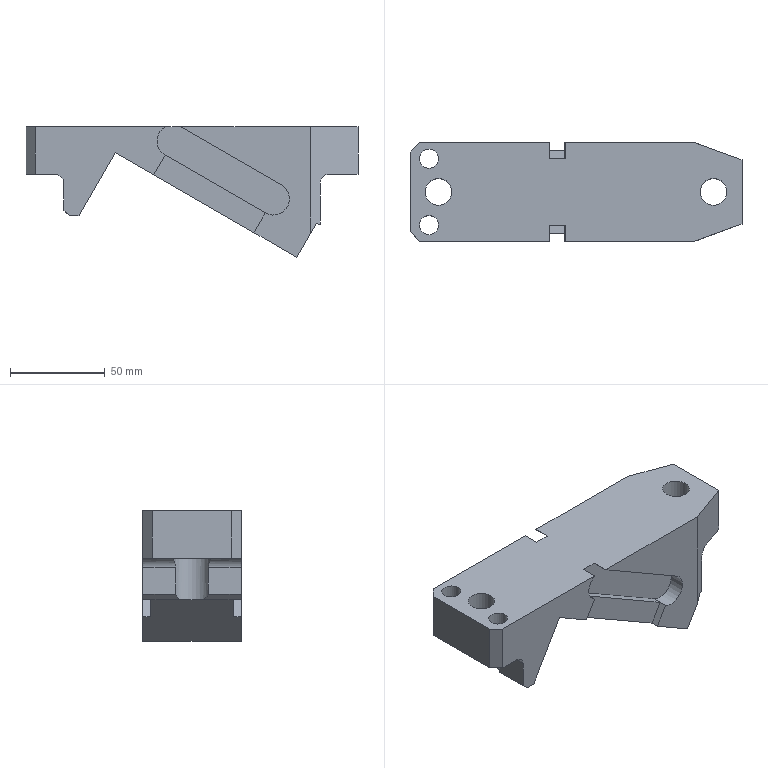Part | NX | features solid 2 | 1 solid | 63 faces | box 175 x 52 x 68.78 mm | volume 293908 mm3 | plane 45 | cylinder 18 | commonest cylinder face diameters 10 x6 17 x6 11 x2 14 x2 20 x2